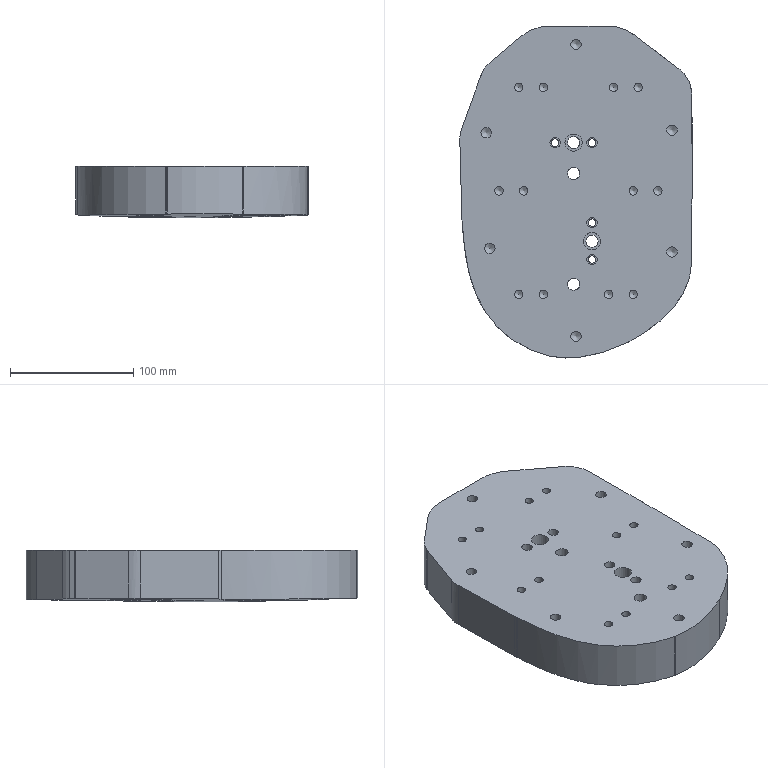Part | STEP file | 415_id1602_x_t | 1 solid | 134 faces | box 188.774 x 269.722 x 41.726 mm | volume 1702520 mm3 | spline 57 | cylinder 38 | cone 22 | plane 15 | sphere 2 | commonest cylinder face diameters 8.5 x14 6.8 x12 6.1 x4 10 x4 14 x2 48.11 x1